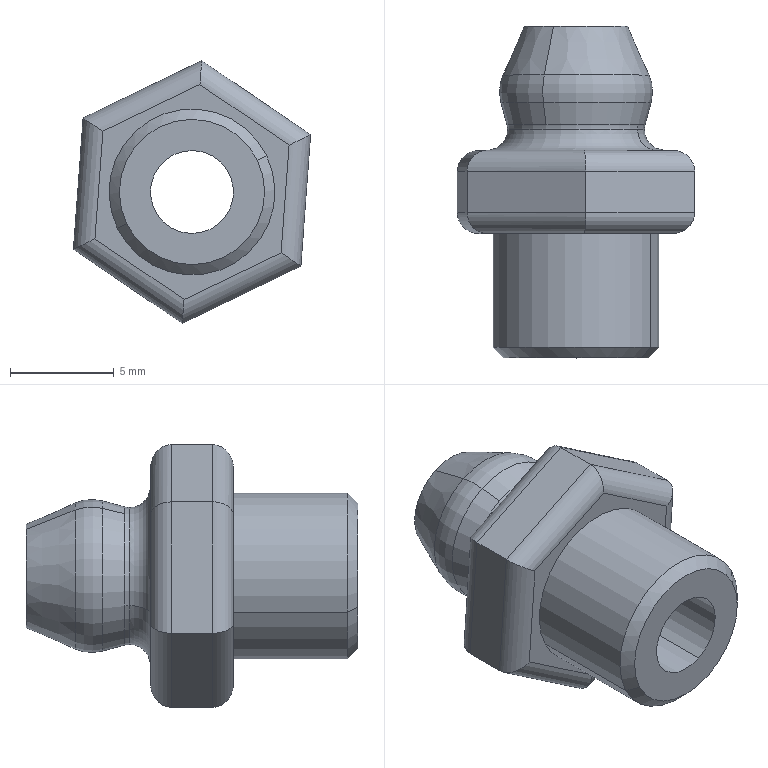Part | STEP file | Input 140 | 1 solid | 38 faces | box 11.44 x 16 x 12.667 mm | volume 712.263 mm3 | cylinder 16 | plane 10 | cone 6 | torus 4 | other 2 | commonest cylinder face diameters 2 x12 4 x2 8 x2